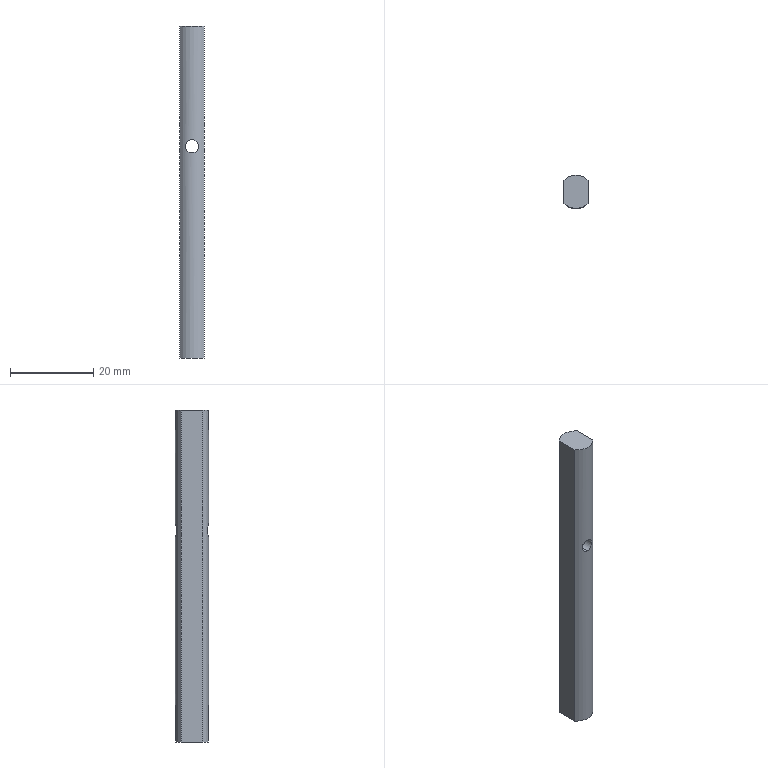Part | STEP file | 8xs200012 | 1 solid | 8 faces | box 6 x 8 x 80 mm | volume 3378 mm3 | cylinder 4 | plane 4 | commonest cylinder face diameters 3.2 x2 8 x2
STEP:
#1=CARTESIAN_POINT('',(0.,0.,0.));
#2=DIRECTION('',(0.,0.,1.));
#3=DIRECTION('',(1.,0.,0.));
#4=AXIS2_PLACEMENT_3D('',#1,#2,#3);
#5=CARTESIAN_POINT('',(0.,-4.,52.6));
#6=VERTEX_POINT('',#5);
#7=CARTESIAN_POINT('',(0.,4.,52.6));
#8=VERTEX_POINT('',#7);
#9=CARTESIAN_POINT('',(0.,-4.,52.6));
#10=DIRECTION('',(0.,1.,0.));
#11=VECTOR('',#10,1.);
#12=LINE('',#9,#11);
#13=CARTESIAN_POINT('',(0.,-4.,51.));
#14=DIRECTION('',(0.,1.,0.));
#15=DIRECTION('',(0.,0.,1.));
#16=AXIS2_PLACEMENT_3D('',#13,#14,#15);
#17=CYLINDRICAL_SURFACE('',#16,1.6);
#18=CARTESIAN_POINT('',(6.283,0.));
#19=DIRECTION('',(0.,1.));
#20=VECTOR('',#19,1.);
#21=LINE('',#18,#20);
#22=(GEOMETRIC_REPRESENTATION_CONTEXT(2)PARAMETRIC_REPRESENTATION_CONTEXT()REPRESENTATION_CONTEXT('',''));
#23=DEFINITIONAL_REPRESENTATION('',(#21),#22);
#24=PCURVE('',#17,#23);
#25=CARTESIAN_POINT('',(0.,-4.,51.));
#26=DIRECTION('',(0.,1.,0.));
#27=DIRECTION('',(0.,0.,1.));
#28=AXIS2_PLACEMENT_3D('',#25,#26,#27);
#29=CYLINDRICAL_SURFACE('',#28,1.6);
#30=CARTESIAN_POINT('',(0.,0.));
#31=DIRECTION('',(0.,1.));
#32=VECTOR('',#31,1.);
#33=LINE('',#30,#32);
#34=(GEOMETRIC_REPRESENTATION_CONTEXT(2)PARAMETRIC_REPRESENTATION_CONTEXT()REPRESENTATION_CONTEXT('',''));
#35=DEFINITIONAL_REPRESENTATION('',(#33),#34);
#36=PCURVE('',#29,#35);
#37=SURFACE_CURVE('',#12,(#24,#36),.PCURVE_S1.);
#38=EDGE_CURVE('',#6,#8,#37,.T.);
#39=ORIENTED_EDGE('',*,*,#38,.T.);
#40=CARTESIAN_POINT('',(0.,4.,49.4));
#41=VERTEX_POINT('',#40);
#42=CARTESIAN_POINT('',(0.,4.,52.6));
#43=CARTESIAN_POINT('',(-0.1069,4.,52.6));
#44=CARTESIAN_POINT('',(-0.2118,3.996,52.589));
#45=CARTESIAN_POINT('',(-0.4179,3.979,52.548));
#46=CARTESIAN_POINT('',(-0.5202,3.967,52.517));
#47=CARTESIAN_POINT('',(-0.8102,3.922,52.396));
#48=CARTESIAN_POINT('',(-0.9862,3.88,52.277));
#49=CARTESIAN_POINT('',(-1.278,3.793,51.985));
#50=CARTESIAN_POINT('',(-1.396,3.749,51.808));
#51=CARTESIAN_POINT('',(-1.517,3.702,51.52));
#52=CARTESIAN_POINT('',(-1.548,3.688,51.418));
#53=CARTESIAN_POINT('',(-1.59,3.671,51.211));
#54=CARTESIAN_POINT('',(-1.6,3.666,51.107));
#55=CARTESIAN_POINT('',(-1.6,3.666,50.895));
#56=CARTESIAN_POINT('',(-1.589,3.671,50.788));
#57=CARTESIAN_POINT('',(-1.548,3.688,50.582));
#58=CARTESIAN_POINT('',(-1.517,3.701,50.481));
#59=CARTESIAN_POINT('',(-1.436,3.734,50.286));
#60=CARTESIAN_POINT('',(-1.387,3.752,50.195));
#61=CARTESIAN_POINT('',(-1.271,3.793,50.023));
#62=CARTESIAN_POINT('',(-1.204,3.815,49.941));
#63=CARTESIAN_POINT('',(-1.058,3.858,49.795));
#64=CARTESIAN_POINT('',(-0.978,3.88,49.729));
#65=CARTESIAN_POINT('',(-0.8051,3.919,49.613));
#66=CARTESIAN_POINT('',(-0.7118,3.937,49.563));
#67=CARTESIAN_POINT('',(-0.4233,3.982,49.443));
#68=CARTESIAN_POINT('',(-0.2106,4.,49.4));
#69=CARTESIAN_POINT('',(0.,4.,49.4));
#70=B_SPLINE_CURVE_WITH_KNOTS('',3,(#42,#43,#44,#45,#46,#47,#48,#49,#50,#51,#52,#53,#54,#55,#56,#57,#58,#59,#60,#61,#62,#63,#64,#65,#66,#67,#68,#69),.UNSPECIFIED.,.F.,.F.,(4,2,2,2,2,2,2,2,2,2,2,2,2,4),(0.,0.000316,0.000632,0.001264,0.001896,0.002212,0.002528,0.002844,0.00316,0.003476,0.003792,0.004108,0.004424,0.005056),.UNSPECIFIED.);
#71=CARTESIAN_POINT('',(6.283,8.));
#72=CARTESIAN_POINT('',(6.267,8.));
#73=CARTESIAN_POINT('',(6.235,7.999));
#74=CARTESIAN_POINT('',(6.187,7.997));
#75=CARTESIAN_POINT('',(6.139,7.994));
#76=CARTESIAN_POINT('',(6.091,7.989));
#77=CARTESIAN_POINT('',(6.043,7.982));
#78=CARTESIAN_POINT('',(5.995,7.974));
#79=CARTESIAN_POINT('',(5.947,7.965));
#80=CARTESIAN_POINT('',(5.899,7.955));
#81=CARTESIAN_POINT('',(5.852,7.944));
#82=CARTESIAN_POINT('',(5.804,7.932));
#83=CARTESIAN_POINT('',(5.757,7.918));
#84=CARTESIAN_POINT('',(5.709,7.905));
#85=CARTESIAN_POINT('',(5.662,7.89));
#86=CARTESIAN_POINT('',(5.615,7.875));
#87=CARTESIAN_POINT('',(5.568,7.86));
#88=CARTESIAN_POINT('',(5.521,7.844));
#89=CARTESIAN_POINT('',(5.474,7.829));
#90=CARTESIAN_POINT('',(5.427,7.813));
#91=CARTESIAN_POINT('',(5.38,7.797));
#92=CARTESIAN_POINT('',(5.332,7.782));
#93=CARTESIAN_POINT('',(5.285,7.767));
#94=CARTESIAN_POINT('',(5.238,7.753));
#95=CARTESIAN_POINT('',(5.19,7.739));
#96=CARTESIAN_POINT('',(5.143,7.726));
#97=CARTESIAN_POINT('',(5.096,7.714));
#98=CARTESIAN_POINT('',(5.048,7.704));
#99=CARTESIAN_POINT('',(5.,7.694));
#100=CARTESIAN_POINT('',(4.952,7.686));
#101=CARTESIAN_POINT('',(4.904,7.678));
#102=CARTESIAN_POINT('',(4.856,7.673));
#103=CARTESIAN_POINT('',(4.809,7.669));
#104=CARTESIAN_POINT('',(4.761,7.667));
#105=CARTESIAN_POINT('',(4.713,7.666));
#106=CARTESIAN_POINT('',(4.665,7.667));
#107=CARTESIAN_POINT('',(4.617,7.669));
#108=CARTESIAN_POINT('',(4.568,7.673));
#109=CARTESIAN_POINT('',(4.52,7.679));
#110=CARTESIAN_POINT('',(4.472,7.686));
#111=CARTESIAN_POINT('',(4.425,7.694));
#112=CARTESIAN_POINT('',(4.377,7.703));
#113=CARTESIAN_POINT('',(4.329,7.714));
#114=CARTESIAN_POINT('',(4.281,7.726));
#115=CARTESIAN_POINT('',(4.234,7.739));
#116=CARTESIAN_POINT('',(4.186,7.753));
#117=CARTESIAN_POINT('',(4.139,7.767));
#118=CARTESIAN_POINT('',(4.092,7.782));
#119=CARTESIAN_POINT('',(4.045,7.797));
#120=CARTESIAN_POINT('',(3.997,7.813));
#121=CARTESIAN_POINT('',(3.95,7.829));
#122=CARTESIAN_POINT('',(3.903,7.845));
#123=CARTESIAN_POINT('',(3.856,7.86));
#124=CARTESIAN_POINT('',(3.809,7.875));
#125=CARTESIAN_POINT('',(3.762,7.89));
#126=CARTESIAN_POINT('',(3.715,7.905));
#127=CARTESIAN_POINT('',(3.667,7.919));
#128=CARTESIAN_POINT('',(3.62,7.932));
#129=CARTESIAN_POINT('',(3.572,7.944));
#130=CARTESIAN_POINT('',(3.525,7.955));
#131=CARTESIAN_POINT('',(3.477,7.965));
#132=CARTESIAN_POINT('',(3.429,7.974));
#133=CARTESIAN_POINT('',(3.382,7.982));
#134=CARTESIAN_POINT('',(3.334,7.988));
#135=CARTESIAN_POINT('',(3.286,7.993));
#136=CARTESIAN_POINT('',(3.238,7.997));
#137=CARTESIAN_POINT('',(3.19,7.999));
#138=CARTESIAN_POINT('',(3.158,8.));
#139=CARTESIAN_POINT('',(3.142,8.));
#140=B_SPLINE_CURVE_WITH_KNOTS('',3,(#71,#72,#73,#74,#75,#76,#77,#78,#79,#80,#81,#82,#83,#84,#85,#86,#87,#88,#89,#90,#91,#92,#93,#94,#95,#96,#97,#98,#99,#100,#101,#102,#103,#104,#105,#106,#107,#108,#109,#110,#111,#112,#113,#114,#115,#116,#117,#118,#119,#120,#121,#122,#123,#124,#125,#126,#127,#128,#129,#130,#131,#132,#133,#134,#135,#136,#137,#138,#139),.UNSPECIFIED.,.F.,.F.,(4,1,1,1,1,1,1,1,1,1,1,1,1,1,1,1,1,1,1,1,1,1,1,1,1,1,1,1,1,1,1,1,1,1,1,1,1,1,1,1,1,1,1,1,1,1,1,1,1,1,1,1,1,1,1,1,1,1,1,1,1,1,1,1,1,1,4),(0.,0.0000766,0.0001532,0.0002298,0.0003064,0.000383,0.0004596,0.0005362,0.0006128,0.0006894,0.000766,0.0008426,0.0009192,0.0009958,0.001072,0.001149,0.001226,0.001302,0.001379,0.001455,0.001532,0.001609,0.001685,0.001762,0.001838,0.001915,0.001992,0.002068,0.002145,0.002221,0.002298,0.002375,0.002451,0.002528,0.002605,0.002681,0.002758,0.002834,0.002911,0.002988,0.003064,0.003141,0.003217,0.003294,0.003371,0.003447,0.003524,0.0036,0.003677,0.003754,0.00383,0.003907,0.003983,0.00406,0.004137,0.004213,0.00429,0.004366,0.004443,0.00452,0.004596,0.004673,0.004749,0.004826,0.004903,0.004979,0.005056),.QUASI_UNIFORM_KNOTS.);
#141=(GEOMETRIC_REPRESENTATION_CONTEXT(2)PARAMETRIC_REPRESENTATION_CONTEXT()REPRESENTATION_CONTEXT('',''));
#142=DEFINITIONAL_REPRESENTATION('',(#140),#141);
#143=PCURVE('',#17,#142);
#144=CARTESIAN_POINT('',(0.,0.,80.));
#145=DIRECTION('',(0.,0.,-1.));
#146=DIRECTION('',(-1.,0.,0.));
#147=AXIS2_PLACEMENT_3D('',#144,#145,#146);
#148=CYLINDRICAL_SURFACE('',#147,4.);
#149=CARTESIAN_POINT('',(1.571,27.4));
#150=CARTESIAN_POINT('',(1.564,27.4));
#151=CARTESIAN_POINT('',(1.551,27.401));
#152=CARTESIAN_POINT('',(1.532,27.407));
#153=CARTESIAN_POINT('',(1.513,27.416));
#154=CARTESIAN_POINT('',(1.494,27.429));
#155=CARTESIAN_POINT('',(1.476,27.445));
#156=CARTESIAN_POINT('',(1.457,27.465));
#157=CARTESIAN_POINT('',(1.438,27.489));
#158=CARTESIAN_POINT('',(1.42,27.516));
#159=CARTESIAN_POINT('',(1.403,27.546));
#160=CARTESIAN_POINT('',(1.385,27.58));
#161=CARTESIAN_POINT('',(1.368,27.616));
#162=CARTESIAN_POINT('',(1.352,27.656));
#163=CARTESIAN_POINT('',(1.336,27.699));
#164=CARTESIAN_POINT('',(1.32,27.744));
#165=CARTESIAN_POINT('',(1.305,27.792));
#166=CARTESIAN_POINT('',(1.291,27.843));
#167=CARTESIAN_POINT('',(1.277,27.896));
#168=CARTESIAN_POINT('',(1.264,27.952));
#169=CARTESIAN_POINT('',(1.251,28.01));
#170=CARTESIAN_POINT('',(1.239,28.07));
#171=CARTESIAN_POINT('',(1.228,28.133));
#172=CARTESIAN_POINT('',(1.217,28.197));
#173=CARTESIAN_POINT('',(1.208,28.264));
#174=CARTESIAN_POINT('',(1.199,28.332));
#175=CARTESIAN_POINT('',(1.191,28.401));
#176=CARTESIAN_POINT('',(1.183,28.472));
#177=CARTESIAN_POINT('',(1.177,28.545));
#178=CARTESIAN_POINT('',(1.172,28.62));
#179=CARTESIAN_POINT('',(1.167,28.695));
#180=CARTESIAN_POINT('',(1.164,28.77));
#181=CARTESIAN_POINT('',(1.161,28.846));
#182=CARTESIAN_POINT('',(1.16,28.922));
#183=CARTESIAN_POINT('',(1.159,28.999));
#184=CARTESIAN_POINT('',(1.16,29.076));
#185=CARTESIAN_POINT('',(1.161,29.153));
#186=CARTESIAN_POINT('',(1.164,29.23));
#187=CARTESIAN_POINT('',(1.167,29.306));
#188=CARTESIAN_POINT('',(1.172,29.38));
#189=CARTESIAN_POINT('',(1.177,29.454));
#190=CARTESIAN_POINT('',(1.183,29.527));
#191=CARTESIAN_POINT('',(1.191,29.599));
#192=CARTESIAN_POINT('',(1.199,29.669));
#193=CARTESIAN_POINT('',(1.208,29.737));
#194=CARTESIAN_POINT('',(1.217,29.804));
#195=CARTESIAN_POINT('',(1.228,29.868));
#196=CARTESIAN_POINT('',(1.239,29.93));
#197=CARTESIAN_POINT('',(1.251,29.991));
#198=CARTESIAN_POINT('',(1.264,30.049));
#199=CARTESIAN_POINT('',(1.277,30.105));
#200=CARTESIAN_POINT('',(1.291,30.159));
#201=CARTESIAN_POINT('',(1.305,30.209));
#202=CARTESIAN_POINT('',(1.32,30.257));
#203=CARTESIAN_POINT('',(1.336,30.302));
#204=CARTESIAN_POINT('',(1.352,30.345));
#205=CARTESIAN_POINT('',(1.369,30.384));
#206=CARTESIAN_POINT('',(1.386,30.421));
#207=CARTESIAN_POINT('',(1.403,30.455));
#208=CARTESIAN_POINT('',(1.421,30.485));
#209=CARTESIAN_POINT('',(1.439,30.511));
#210=CARTESIAN_POINT('',(1.457,30.535));
#211=CARTESIAN_POINT('',(1.476,30.554));
#212=CARTESIAN_POINT('',(1.494,30.571));
#213=CARTESIAN_POINT('',(1.513,30.584));
#214=CARTESIAN_POINT('',(1.532,30.593));
#215=CARTESIAN_POINT('',(1.552,30.599));
#216=CARTESIAN_POINT('',(1.564,30.6));
#217=CARTESIAN_POINT('',(1.571,30.6));
#218=B_SPLINE_CURVE_WITH_KNOTS('',3,(#149,#150,#151,#152,#153,#154,#155,#156,#157,#158,#159,#160,#161,#162,#163,#164,#165,#166,#167,#168,#169,#170,#171,#172,#173,#174,#175,#176,#177,#178,#179,#180,#181,#182,#183,#184,#185,#186,#187,#188,#189,#190,#191,#192,#193,#194,#195,#196,#197,#198,#199,#200,#201,#202,#203,#204,#205,#206,#207,#208,#209,#210,#211,#212,#213,#214,#215,#216,#217),.UNSPECIFIED.,.F.,.F.,(4,1,1,1,1,1,1,1,1,1,1,1,1,1,1,1,1,1,1,1,1,1,1,1,1,1,1,1,1,1,1,1,1,1,1,1,1,1,1,1,1,1,1,1,1,1,1,1,1,1,1,1,1,1,1,1,1,1,1,1,1,1,1,1,1,1,4),(0.,0.0000766,0.0001532,0.0002298,0.0003064,0.000383,0.0004596,0.0005362,0.0006128,0.0006894,0.000766,0.0008426,0.0009192,0.0009958,0.001072,0.001149,0.001226,0.001302,0.001379,0.001455,0.001532,0.001609,0.001685,0.001762,0.001838,0.001915,0.001992,0.002068,0.002145,0.002221,0.002298,0.002375,0.002451,0.002528,0.002605,0.002681,0.002758,0.002834,0.002911,0.002988,0.003064,0.003141,0.003217,0.003294,0.003371,0.003447,0.003524,0.0036,0.003677,0.003754,0.00383,0.003907,0.003983,0.00406,0.004137,0.004213,0.00429,0.004366,0.004443,0.00452,0.004596,0.004673,0.004749,0.004826,0.004903,0.004979,0.005056),.QUASI_UNIFORM_KNOTS.);
#219=(GEOMETRIC_REPRESENTATION_CONTEXT(2)PARAMETRIC_REPRESENTATION_CONTEXT()REPRESENTATION_CONTEXT('',''));
#220=DEFINITIONAL_REPRESENTATION('',(#218),#219);
#221=PCURVE('',#148,#220);
#222=SURFACE_CURVE('',#70,(#143,#221),.PCURVE_S1.);
#223=EDGE_CURVE('',#8,#41,#222,.T.);
#224=ORIENTED_EDGE('',*,*,#223,.T.);
#225=CARTESIAN_POINT('',(0.,-4.,49.4));
#226=VERTEX_POINT('',#225);
#227=CARTESIAN_POINT('',(0.,-4.,49.4));
#228=DIRECTION('',(0.,1.,0.));
#229=VECTOR('',#228,1.);
#230=LINE('',#227,#229);
#231=CARTESIAN_POINT('',(3.142,0.));
#232=DIRECTION('',(0.,1.));
#233=VECTOR('',#232,1.);
#234=LINE('',#231,#233);
#235=(GEOMETRIC_REPRESENTATION_CONTEXT(2)PARAMETRIC_REPRESENTATION_CONTEXT()REPRESENTATION_CONTEXT('',''));
#236=DEFINITIONAL_REPRESENTATION('',(#234),#235);
#237=PCURVE('',#17,#236);
#238=CARTESIAN_POINT('',(3.142,0.));
#239=DIRECTION('',(0.,1.));
#240=VECTOR('',#239,1.);
#241=LINE('',#238,#240);
#242=(GEOMETRIC_REPRESENTATION_CONTEXT(2)PARAMETRIC_REPRESENTATION_CONTEXT()REPRESENTATION_CONTEXT('',''));
#243=DEFINITIONAL_REPRESENTATION('',(#241),#242);
#244=PCURVE('',#29,#243);
#245=SURFACE_CURVE('',#230,(#237,#244),.PCURVE_S1.);
#246=EDGE_CURVE('',#226,#41,#245,.T.);
#247=ORIENTED_EDGE('',*,*,#246,.F.);
#248=CARTESIAN_POINT('',(0.,-4.,49.4));
#249=CARTESIAN_POINT('',(-0.1052,-4.,49.4));
#250=CARTESIAN_POINT('',(-0.2119,-3.996,49.411));
#251=CARTESIAN_POINT('',(-0.4193,-3.979,49.452));
#252=CARTESIAN_POINT('',(-0.5194,-3.967,49.483));
#253=CARTESIAN_POINT('',(-0.713,-3.937,49.564));
#254=CARTESIAN_POINT('',(-0.8061,-3.919,49.614));
#255=CARTESIAN_POINT('',(-0.9782,-3.88,49.73));
#256=CARTESIAN_POINT('',(-1.058,-3.858,49.796));
#257=CARTESIAN_POINT('',(-1.206,-3.815,49.943));
#258=CARTESIAN_POINT('',(-1.271,-3.793,50.023));
#259=CARTESIAN_POINT('',(-1.387,-3.752,50.195));
#260=CARTESIAN_POINT('',(-1.437,-3.733,50.288));
#261=CARTESIAN_POINT('',(-1.517,-3.701,50.481));
#262=CARTESIAN_POINT('',(-1.548,-3.689,50.581));
#263=CARTESIAN_POINT('',(-1.589,-3.671,50.787));
#264=CARTESIAN_POINT('',(-1.6,-3.666,50.894));
#265=CARTESIAN_POINT('',(-1.6,-3.666,51.211));
#266=CARTESIAN_POINT('',(-1.557,-3.685,51.423));
#267=CARTESIAN_POINT('',(-1.437,-3.733,51.712));
#268=CARTESIAN_POINT('',(-1.387,-3.752,51.805));
#269=CARTESIAN_POINT('',(-1.271,-3.793,51.978));
#270=CARTESIAN_POINT('',(-1.205,-3.815,52.057));
#271=CARTESIAN_POINT('',(-1.059,-3.858,52.204));
#272=CARTESIAN_POINT('',(-0.9774,-3.88,52.271));
#273=CARTESIAN_POINT('',(-0.8055,-3.919,52.386));
#274=CARTESIAN_POINT('',(-0.7141,-3.937,52.436));
#275=CARTESIAN_POINT('',(-0.4218,-3.983,52.558));
#276=CARTESIAN_POINT('',(-0.2137,-4.,52.6));
#277=CARTESIAN_POINT('',(0.,-4.,52.6));
#278=B_SPLINE_CURVE_WITH_KNOTS('',3,(#248,#249,#250,#251,#252,#253,#254,#255,#256,#257,#258,#259,#260,#261,#262,#263,#264,#265,#266,#267,#268,#269,#270,#271,#272,#273,#274,#275,#276,#277),.UNSPECIFIED.,.F.,.F.,(4,2,2,2,2,2,2,2,2,2,2,2,2,2,4),(0.005056,0.005372,0.005687,0.006003,0.006319,0.006635,0.006951,0.007266,0.007582,0.008214,0.008529,0.008845,0.009161,0.009477,0.01011),.UNSPECIFIED.);
#279=CARTESIAN_POINT('',(3.142,0.));
#280=CARTESIAN_POINT('',(3.158,0.));
#281=CARTESIAN_POINT('',(3.19,0.0005013));
#282=CARTESIAN_POINT('',(3.238,0.00273));
#283=CARTESIAN_POINT('',(3.286,0.006405));
#284=CARTESIAN_POINT('',(3.334,0.01151));
#285=CARTESIAN_POINT('',(3.382,0.01798));
#286=CARTESIAN_POINT('',(3.43,0.02573));
#287=CARTESIAN_POINT('',(3.477,0.03471));
#288=CARTESIAN_POINT('',(3.525,0.04485));
#289=CARTESIAN_POINT('',(3.573,0.05611));
#290=CARTESIAN_POINT('',(3.62,0.06838));
#291=CARTESIAN_POINT('',(3.668,0.0815));
#292=CARTESIAN_POINT('',(3.715,0.09534));
#293=CARTESIAN_POINT('',(3.763,0.1097));
#294=CARTESIAN_POINT('',(3.81,0.1247));
#295=CARTESIAN_POINT('',(3.857,0.14));
#296=CARTESIAN_POINT('',(3.904,0.1556));
#297=CARTESIAN_POINT('',(3.951,0.1715));
#298=CARTESIAN_POINT('',(3.999,0.1872));
#299=CARTESIAN_POINT('',(4.046,0.2028));
#300=CARTESIAN_POINT('',(4.092,0.218));
#301=CARTESIAN_POINT('',(4.139,0.2328));
#302=CARTESIAN_POINT('',(4.187,0.2472));
#303=CARTESIAN_POINT('',(4.234,0.2609));
#304=CARTESIAN_POINT('',(4.282,0.2738));
#305=CARTESIAN_POINT('',(4.329,0.2857));
#306=CARTESIAN_POINT('',(4.377,0.2965));
#307=CARTESIAN_POINT('',(4.424,0.3061));
#308=CARTESIAN_POINT('',(4.472,0.3144));
#309=CARTESIAN_POINT('',(4.519,0.3214));
#310=CARTESIAN_POINT('',(4.568,0.3269));
#311=CARTESIAN_POINT('',(4.616,0.3309));
#312=CARTESIAN_POINT('',(4.664,0.3334));
#313=CARTESIAN_POINT('',(4.712,0.3342));
#314=CARTESIAN_POINT('',(4.76,0.3334));
#315=CARTESIAN_POINT('',(4.808,0.3309));
#316=CARTESIAN_POINT('',(4.856,0.3268));
#317=CARTESIAN_POINT('',(4.904,0.3213));
#318=CARTESIAN_POINT('',(4.952,0.3143));
#319=CARTESIAN_POINT('',(5.,0.306));
#320=CARTESIAN_POINT('',(5.048,0.2964));
#321=CARTESIAN_POINT('',(5.095,0.2857));
#322=CARTESIAN_POINT('',(5.143,0.2738));
#323=CARTESIAN_POINT('',(5.191,0.2609));
#324=CARTESIAN_POINT('',(5.238,0.2471));
#325=CARTESIAN_POINT('',(5.286,0.2327));
#326=CARTESIAN_POINT('',(5.333,0.2178));
#327=CARTESIAN_POINT('',(5.38,0.2026));
#328=CARTESIAN_POINT('',(5.427,0.1871));
#329=CARTESIAN_POINT('',(5.474,0.1714));
#330=CARTESIAN_POINT('',(5.521,0.1556));
#331=CARTESIAN_POINT('',(5.568,0.1399));
#332=CARTESIAN_POINT('',(5.616,0.1245));
#333=CARTESIAN_POINT('',(5.663,0.1096));
#334=CARTESIAN_POINT('',(5.71,0.09517));
#335=CARTESIAN_POINT('',(5.757,0.08144));
#336=CARTESIAN_POINT('',(5.804,0.06843));
#337=CARTESIAN_POINT('',(5.852,0.05623));
#338=CARTESIAN_POINT('',(5.9,0.0449));
#339=CARTESIAN_POINT('',(5.947,0.03471));
#340=CARTESIAN_POINT('',(5.995,0.02572));
#341=CARTESIAN_POINT('',(6.043,0.01799));
#342=CARTESIAN_POINT('',(6.091,0.01155));
#343=CARTESIAN_POINT('',(6.139,0.006464));
#344=CARTESIAN_POINT('',(6.187,0.002767));
#345=CARTESIAN_POINT('',(6.235,0.0005118));
#346=CARTESIAN_POINT('',(6.267,0.));
#347=CARTESIAN_POINT('',(6.283,0.));
#348=B_SPLINE_CURVE_WITH_KNOTS('',3,(#279,#280,#281,#282,#283,#284,#285,#286,#287,#288,#289,#290,#291,#292,#293,#294,#295,#296,#297,#298,#299,#300,#301,#302,#303,#304,#305,#306,#307,#308,#309,#310,#311,#312,#313,#314,#315,#316,#317,#318,#319,#320,#321,#322,#323,#324,#325,#326,#327,#328,#329,#330,#331,#332,#333,#334,#335,#336,#337,#338,#339,#340,#341,#342,#343,#344,#345,#346,#347),.UNSPECIFIED.,.F.,.F.,(4,1,1,1,1,1,1,1,1,1,1,1,1,1,1,1,1,1,1,1,1,1,1,1,1,1,1,1,1,1,1,1,1,1,1,1,1,1,1,1,1,1,1,1,1,1,1,1,1,1,1,1,1,1,1,1,1,1,1,1,1,1,1,1,1,1,4),(0.005056,0.005132,0.005209,0.005285,0.005362,0.005439,0.005515,0.005592,0.005668,0.005745,0.005821,0.005898,0.005974,0.006051,0.006128,0.006204,0.006281,0.006357,0.006434,0.00651,0.006587,0.006663,0.00674,0.006817,0.006893,0.00697,0.007046,0.007123,0.007199,0.007276,0.007352,0.007429,0.007506,0.007582,0.007659,0.007735,0.007812,0.007888,0.007965,0.008041,0.008118,0.008195,0.008271,0.008348,0.008424,0.008501,0.008577,0.008654,0.00873,0.008807,0.008883,0.00896,0.009037,0.009113,0.00919,0.009266,0.009343,0.009419,0.009496,0.009572,0.009649,0.009726,0.009802,0.009879,0.009955,0.01003,0.01011),.QUASI_UNIFORM_KNOTS.);
#349=(GEOMETRIC_REPRESENTATION_CONTEXT(2)PARAMETRIC_REPRESENTATION_CONTEXT()REPRESENTATION_CONTEXT('',''));
#350=DEFINITIONAL_REPRESENTATION('',(#348),#349);
#351=PCURVE('',#17,#350);
#352=CARTESIAN_POINT('',(0.,0.,80.));
#353=DIRECTION('',(0.,0.,-1.));
#354=DIRECTION('',(-1.,0.,0.));
#355=AXIS2_PLACEMENT_3D('',#352,#353,#354);
#356=CYLINDRICAL_SURFACE('',#355,4.);
#357=CARTESIAN_POINT('',(4.712,30.6));
#358=CARTESIAN_POINT('',(4.719,30.6));
#359=CARTESIAN_POINT('',(4.732,30.599));
#360=CARTESIAN_POINT('',(4.751,30.593));
#361=CARTESIAN_POINT('',(4.77,30.584));
#362=CARTESIAN_POINT('',(4.789,30.571));
#363=CARTESIAN_POINT('',(4.808,30.555));
#364=CARTESIAN_POINT('',(4.826,30.535));
#365=CARTESIAN_POINT('',(4.845,30.511));
#366=CARTESIAN_POINT('',(4.863,30.484));
#367=CARTESIAN_POINT('',(4.88,30.454));
#368=CARTESIAN_POINT('',(4.898,30.421));
#369=CARTESIAN_POINT('',(4.915,30.384));
#370=CARTESIAN_POINT('',(4.931,30.344));
#371=CARTESIAN_POINT('',(4.947,30.302));
#372=CARTESIAN_POINT('',(4.963,30.257));
#373=CARTESIAN_POINT('',(4.978,30.208));
#374=CARTESIAN_POINT('',(4.992,30.158));
#375=CARTESIAN_POINT('',(5.006,30.104));
#376=CARTESIAN_POINT('',(5.02,30.048));
#377=CARTESIAN_POINT('',(5.032,29.99));
#378=CARTESIAN_POINT('',(5.044,29.93));
#379=CARTESIAN_POINT('',(5.055,29.868));
#380=CARTESIAN_POINT('',(5.066,29.803));
#381=CARTESIAN_POINT('',(5.076,29.736));
#382=CARTESIAN_POINT('',(5.085,29.668));
#383=CARTESIAN_POINT('',(5.093,29.598));
#384=CARTESIAN_POINT('',(5.1,29.527));
#385=CARTESIAN_POINT('',(5.106,29.455));
#386=CARTESIAN_POINT('',(5.112,29.381));
#387=CARTESIAN_POINT('',(5.116,29.307));
#388=CARTESIAN_POINT('',(5.119,29.231));
#389=CARTESIAN_POINT('',(5.122,29.154));
#390=CARTESIAN_POINT('',(5.124,29.077));
#391=CARTESIAN_POINT('',(5.124,29.));
#392=CARTESIAN_POINT('',(5.124,28.923));
#393=CARTESIAN_POINT('',(5.122,28.847));
#394=CARTESIAN_POINT('',(5.119,28.771));
#395=CARTESIAN_POINT('',(5.116,28.695));
#396=CARTESIAN_POINT('',(5.112,28.62));
#397=CARTESIAN_POINT('',(5.106,28.546));
#398=CARTESIAN_POINT('',(5.1,28.473));
#399=CARTESIAN_POINT('',(5.093,28.402));
#400=CARTESIAN_POINT('',(5.085,28.332));
#401=CARTESIAN_POINT('',(5.076,28.264));
#402=CARTESIAN_POINT('',(5.066,28.197));
#403=CARTESIAN_POINT('',(5.055,28.132));
#404=CARTESIAN_POINT('',(5.044,28.069));
#405=CARTESIAN_POINT('',(5.032,28.009));
#406=CARTESIAN_POINT('',(5.02,27.951));
#407=CARTESIAN_POINT('',(5.006,27.896));
#408=CARTESIAN_POINT('',(4.992,27.842));
#409=CARTESIAN_POINT('',(4.978,27.791));
#410=CARTESIAN_POINT('',(4.963,27.743));
#411=CARTESIAN_POINT('',(4.947,27.698));
#412=CARTESIAN_POINT('',(4.931,27.655));
#413=CARTESIAN_POINT('',(4.915,27.616));
#414=CARTESIAN_POINT('',(4.898,27.58));
#415=CARTESIAN_POINT('',(4.881,27.546));
#416=CARTESIAN_POINT('',(4.863,27.516));
#417=CARTESIAN_POINT('',(4.845,27.489));
#418=CARTESIAN_POINT('',(4.826,27.465));
#419=CARTESIAN_POINT('',(4.808,27.445));
#420=CARTESIAN_POINT('',(4.789,27.429));
#421=CARTESIAN_POINT('',(4.77,27.416));
#422=CARTESIAN_POINT('',(4.751,27.407));
#423=CARTESIAN_POINT('',(4.732,27.401));
#424=CARTESIAN_POINT('',(4.719,27.4));
#425=CARTESIAN_POINT('',(4.712,27.4));
#426=B_SPLINE_CURVE_WITH_KNOTS('',3,(#357,#358,#359,#360,#361,#362,#363,#364,#365,#366,#367,#368,#369,#370,#371,#372,#373,#374,#375,#376,#377,#378,#379,#380,#381,#382,#383,#384,#385,#386,#387,#388,#389,#390,#391,#392,#393,#394,#395,#396,#397,#398,#399,#400,#401,#402,#403,#404,#405,#406,#407,#408,#409,#410,#411,#412,#413,#414,#415,#416,#417,#418,#419,#420,#421,#422,#423,#424,#425),.UNSPECIFIED.,.F.,.F.,(4,1,1,1,1,1,1,1,1,1,1,1,1,1,1,1,1,1,1,1,1,1,1,1,1,1,1,1,1,1,1,1,1,1,1,1,1,1,1,1,1,1,1,1,1,1,1,1,1,1,1,1,1,1,1,1,1,1,1,1,1,1,1,1,1,1,4),(0.005056,0.005132,0.005209,0.005285,0.005362,0.005439,0.005515,0.005592,0.005668,0.005745,0.005821,0.005898,0.005974,0.006051,0.006128,0.006204,0.006281,0.006357,0.006434,0.00651,0.006587,0.006663,0.00674,0.006817,0.006893,0.00697,0.007046,0.007123,0.007199,0.007276,0.007352,0.007429,0.007506,0.007582,0.007659,0.007735,0.007812,0.007888,0.007965,0.008041,0.008118,0.008195,0.008271,0.008348,0.008424,0.008501,0.008577,0.008654,0.00873,0.008807,0.008883,0.00896,0.009037,0.009113,0.00919,0.009266,0.009343,0.009419,0.009496,0.009572,0.009649,0.009726,0.009802,0.009879,0.009955,0.01003,0.01011),.QUASI_UNIFORM_KNOTS.);
#427=(GEOMETRIC_REPRESENTATION_CONTEXT(2)PARAMETRIC_REPRESENTATION_CONTEXT()REPRESENTATION_CONTEXT('',''));
#428=DEFINITIONAL_REPRESENTATION('',(#426),#427);
#429=PCURVE('',#356,#428);
#430=SURFACE_CURVE('',#278,(#351,#429),.PCURVE_S1.);
#431=EDGE_CURVE('',#226,#6,#430,.T.);
#432=ORIENTED_EDGE('',*,*,#431,.T.);
#433=EDGE_LOOP('',(#39,#224,#247,#432));
#434=FACE_BOUND('',#433,.F.);
#435=ADVANCED_FACE('',(#434),#17,.F.);
#436=ORIENTED_EDGE('',*,*,#223,.T.);
#437=CARTESIAN_POINT('',(0.,4.,49.4));
#438=CARTESIAN_POINT('',(0.1052,4.,49.4));
#439=CARTESIAN_POINT('',(0.2119,3.996,49.411));
#440=CARTESIAN_POINT('',(0.4193,3.979,49.452));
#441=CARTESIAN_POINT('',(0.5194,3.967,49.483));
#442=CARTESIAN_POINT('',(0.713,3.937,49.564));
#443=CARTESIAN_POINT('',(0.8061,3.919,49.614));
#444=CARTESIAN_POINT('',(0.9782,3.88,49.73));
#445=CARTESIAN_POINT('',(1.058,3.858,49.796));
#446=CARTESIAN_POINT('',(1.206,3.815,49.943));
#447=CARTESIAN_POINT('',(1.271,3.793,50.023));
#448=CARTESIAN_POINT('',(1.387,3.752,50.195));
#449=CARTESIAN_POINT('',(1.437,3.733,50.288));
#450=CARTESIAN_POINT('',(1.517,3.701,50.481));
#451=CARTESIAN_POINT('',(1.548,3.689,50.581));
#452=CARTESIAN_POINT('',(1.589,3.671,50.787));
#453=CARTESIAN_POINT('',(1.6,3.666,50.894));
#454=CARTESIAN_POINT('',(1.6,3.666,51.211));
#455=CARTESIAN_POINT('',(1.557,3.685,51.423));
#456=CARTESIAN_POINT('',(1.437,3.733,51.712));
#457=CARTESIAN_POINT('',(1.387,3.752,51.805));
#458=CARTESIAN_POINT('',(1.271,3.793,51.978));
#459=CARTESIAN_POINT('',(1.205,3.815,52.057));
#460=CARTESIAN_POINT('',(1.059,3.858,52.204));
#461=CARTESIAN_POINT('',(0.9774,3.88,52.271));
#462=CARTESIAN_POINT('',(0.8055,3.919,52.386));
#463=CARTESIAN_POINT('',(0.7141,3.937,52.436));
#464=CARTESIAN_POINT('',(0.4218,3.983,52.558));
#465=CARTESIAN_POINT('',(0.2137,4.,52.6));
#466=CARTESIAN_POINT('',(0.,4.,52.6));
#467=B_SPLINE_CURVE_WITH_KNOTS('',3,(#437,#438,#439,#440,#441,#442,#443,#444,#445,#446,#447,#448,#449,#450,#451,#452,#453,#454,#455,#456,#457,#458,#459,#460,#461,#462,#463,#464,#465,#466),.UNSPECIFIED.,.F.,.F.,(4,2,2,2,2,2,2,2,2,2,2,2,2,2,4),(0.005056,0.005372,0.005687,0.006003,0.006319,0.006635,0.006951,0.007266,0.007582,0.008214,0.008529,0.008845,0.009161,0.009477,0.01011),.UNSPECIFIED.);
#468=CARTESIAN_POINT('',(1.571,30.6));
#469=CARTESIAN_POINT('',(1.577,30.6));
#470=CARTESIAN_POINT('',(1.59,30.599));
#471=CARTESIAN_POINT('',(1.609,30.593));
#472=CARTESIAN_POINT('',(1.628,30.584));
#473=CARTESIAN_POINT('',(1.647,30.571));
#474=CARTESIAN_POINT('',(1.666,30.555));
#475=CARTESIAN_POINT('',(1.685,30.535));
#476=CARTESIAN_POINT('',(1.703,30.511));
#477=CARTESIAN_POINT('',(1.721,30.484));
#478=CARTESIAN_POINT('',(1.739,30.454));
#479=CARTESIAN_POINT('',(1.756,30.421));
#480=CARTESIAN_POINT('',(1.773,30.384));
#481=CARTESIAN_POINT('',(1.79,30.344));
#482=CARTESIAN_POINT('',(1.806,30.302));
#483=CARTESIAN_POINT('',(1.821,30.257));
#484=CARTESIAN_POINT('',(1.836,30.208));
#485=CARTESIAN_POINT('',(1.851,30.158));
#486=CARTESIAN_POINT('',(1.865,30.104));
#487=CARTESIAN_POINT('',(1.878,30.048));
#488=CARTESIAN_POINT('',(1.891,29.99));
#489=CARTESIAN_POINT('',(1.903,29.93));
#490=CARTESIAN_POINT('',(1.914,29.868));
#491=CARTESIAN_POINT('',(1.924,29.803));
#492=CARTESIAN_POINT('',(1.934,29.736));
#493=CARTESIAN_POINT('',(1.943,29.668));
#494=CARTESIAN_POINT('',(1.951,29.598));
#495=CARTESIAN_POINT('',(1.958,29.527));
#496=CARTESIAN_POINT('',(1.965,29.455));
#497=CARTESIAN_POINT('',(1.97,29.381));
#498=CARTESIAN_POINT('',(1.974,29.307));
#499=CARTESIAN_POINT('',(1.978,29.231));
#500=CARTESIAN_POINT('',(1.98,29.154));
#501=CARTESIAN_POINT('',(1.982,29.077));
#502=CARTESIAN_POINT('',(1.982,29.));
#503=CARTESIAN_POINT('',(1.982,28.923));
#504=CARTESIAN_POINT('',(1.98,28.847));
#505=CARTESIAN_POINT('',(1.978,28.771));
#506=CARTESIAN_POINT('',(1.974,28.695));
#507=CARTESIAN_POINT('',(1.97,28.62));
#508=CARTESIAN_POINT('',(1.965,28.546));
#509=CARTESIAN_POINT('',(1.958,28.473));
#510=CARTESIAN_POINT('',(1.951,28.402));
#511=CARTESIAN_POINT('',(1.943,28.332));
#512=CARTESIAN_POINT('',(1.934,28.264));
#513=CARTESIAN_POINT('',(1.924,28.197));
#514=CARTESIAN_POINT('',(1.914,28.132));
#515=CARTESIAN_POINT('',(1.902,28.069));
#516=CARTESIAN_POINT('',(1.89,28.009));
#517=CARTESIAN_POINT('',(1.878,27.951));
#518=CARTESIAN_POINT('',(1.865,27.896));
#519=CARTESIAN_POINT('',(1.851,27.842));
#520=CARTESIAN_POINT('',(1.836,27.791));
#521=CARTESIAN_POINT('',(1.821,27.743));
#522=CARTESIAN_POINT('',(1.806,27.698));
#523=CARTESIAN_POINT('',(1.79,27.655));
#524=CARTESIAN_POINT('',(1.773,27.616));
#525=CARTESIAN_POINT('',(1.756,27.58));
#526=CARTESIAN_POINT('',(1.739,27.546));
#527=CARTESIAN_POINT('',(1.721,27.516));
#528=CARTESIAN_POINT('',(1.703,27.489));
#529=CARTESIAN_POINT('',(1.685,27.465));
#530=CARTESIAN_POINT('',(1.666,27.445));
#531=CARTESIAN_POINT('',(1.647,27.429));
#532=CARTESIAN_POINT('',(1.628,27.416));
#533=CARTESIAN_POINT('',(1.609,27.407));
#534=CARTESIAN_POINT('',(1.59,27.401));
#535=CARTESIAN_POINT('',(1.577,27.4));
#536=CARTESIAN_POINT('',(1.571,27.4));
#537=B_SPLINE_CURVE_WITH_KNOTS('',3,(#468,#469,#470,#471,#472,#473,#474,#475,#476,#477,#478,#479,#480,#481,#482,#483,#484,#485,#486,#487,#488,#489,#490,#491,#492,#493,#494,#495,#496,#497,#498,#499,#500,#501,#502,#503,#504,#505,#506,#507,#508,#509,#510,#511,#512,#513,#514,#515,#516,#517,#518,#519,#520,#521,#522,#523,#524,#525,#526,#527,#528,#529,#530,#531,#532,#533,#534,#535,#536),.UNSPECIFIED.,.F.,.F.,(4,1,1,1,1,1,1,1,1,1,1,1,1,1,1,1,1,1,1,1,1,1,1,1,1,1,1,1,1,1,1,1,1,1,1,1,1,1,1,1,1,1,1,1,1,1,1,1,1,1,1,1,1,1,1,1,1,1,1,1,1,1,1,1,1,1,4),(0.005056,0.005132,0.005209,0.005285,0.005362,0.005439,0.005515,0.005592,0.005668,0.005745,0.005821,0.005898,0.005974,0.006051,0.006128,0.006204,0.006281,0.006357,0.006434,0.00651,0.006587,0.006663,0.00674,0.006817,0.006893,0.00697,0.007046,0.007123,0.007199,0.007276,0.007352,0.007429,0.007506,0.007582,0.007659,0.007735,0.007812,0.007888,0.007965,0.008041,0.008118,0.008195,0.008271,0.008348,0.008424,0.008501,0.008577,0.008654,0.00873,0.008807,0.008883,0.00896,0.009037,0.009113,0.00919,0.009266,0.009343,0.009419,0.009496,0.009572,0.009649,0.009726,0.009802,0.009879,0.009955,0.01003,0.01011),.QUASI_UNIFORM_KNOTS.);
#538=(GEOMETRIC_REPRESENTATION_CONTEXT(2)PARAMETRIC_REPRESENTATION_CONTEXT()REPRESENTATION_CONTEXT('',''));
#539=DEFINITIONAL_REPRESENTATION('',(#537),#538);
#540=PCURVE('',#148,#539);
#541=CARTESIAN_POINT('',(3.142,8.));
#542=CARTESIAN_POINT('',(3.126,8.));
#543=CARTESIAN_POINT('',(3.094,7.999));
#544=CARTESIAN_POINT('',(3.045,7.997));
#545=CARTESIAN_POINT('',(2.997,7.994));
#546=CARTESIAN_POINT('',(2.949,7.988));
#547=CARTESIAN_POINT('',(2.901,7.982));
#548=CARTESIAN_POINT('',(2.853,7.974));
#549=CARTESIAN_POINT('',(2.806,7.965));
#550=CARTESIAN_POINT('',(2.758,7.955));
#551=CARTESIAN_POINT('',(2.71,7.944));
#552=CARTESIAN_POINT('',(2.663,7.932));
#553=CARTESIAN_POINT('',(2.615,7.918));
#554=CARTESIAN_POINT('',(2.568,7.905));
#555=CARTESIAN_POINT('',(2.521,7.89));
#556=CARTESIAN_POINT('',(2.474,7.875));
#557=CARTESIAN_POINT('',(2.426,7.86));
#558=CARTESIAN_POINT('',(2.379,7.844));
#559=CARTESIAN_POINT('',(2.332,7.828));
#560=CARTESIAN_POINT('',(2.285,7.813));
#561=CARTESIAN_POINT('',(2.238,7.797));
#562=CARTESIAN_POINT('',(2.191,7.782));
#563=CARTESIAN_POINT('',(2.144,7.767));
#564=CARTESIAN_POINT('',(2.096,7.753));
#565=CARTESIAN_POINT('',(2.049,7.739));
#566=CARTESIAN_POINT('',(2.001,7.726));
#567=CARTESIAN_POINT('',(1.954,7.714));
#568=CARTESIAN_POINT('',(1.906,7.704));
#569=CARTESIAN_POINT('',(1.859,7.694));
#570=CARTESIAN_POINT('',(1.811,7.686));
#571=CARTESIAN_POINT('',(1.764,7.679));
#572=CARTESIAN_POINT('',(1.716,7.673));
#573=CARTESIAN_POINT('',(1.667,7.669));
#574=CARTESIAN_POINT('',(1.619,7.667));
#575=CARTESIAN_POINT('',(1.571,7.666));
#576=CARTESIAN_POINT('',(1.523,7.667));
#577=CARTESIAN_POINT('',(1.475,7.669));
#578=CARTESIAN_POINT('',(1.427,7.673));
#579=CARTESIAN_POINT('',(1.379,7.679));
#580=CARTESIAN_POINT('',(1.331,7.686));
#581=CARTESIAN_POINT('',(1.283,7.694));
#582=CARTESIAN_POINT('',(1.235,7.704));
#583=CARTESIAN_POINT('',(1.188,7.714));
#584=CARTESIAN_POINT('',(1.14,7.726));
#585=CARTESIAN_POINT('',(1.093,7.739));
#586=CARTESIAN_POINT('',(1.045,7.753));
#587=CARTESIAN_POINT('',(0.9976,7.767));
#588=CARTESIAN_POINT('',(0.9504,7.782));
#589=CARTESIAN_POINT('',(0.9034,7.797));
#590=CARTESIAN_POINT('',(0.8564,7.813));
#591=CARTESIAN_POINT('',(0.8094,7.829));
#592=CARTESIAN_POINT('',(0.7623,7.844));
#593=CARTESIAN_POINT('',(0.7149,7.86));
#594=CARTESIAN_POINT('',(0.6676,7.875));
#595=CARTESIAN_POINT('',(0.6203,7.89));
#596=CARTESIAN_POINT('',(0.5733,7.905));
#597=CARTESIAN_POINT('',(0.5263,7.919));
#598=CARTESIAN_POINT('',(0.479,7.932));
#599=CARTESIAN_POINT('',(0.4316,7.944));
#600=CARTESIAN_POINT('',(0.3836,7.955));
#601=CARTESIAN_POINT('',(0.3357,7.965));
#602=CARTESIAN_POINT('',(0.288,7.974));
#603=CARTESIAN_POINT('',(0.2402,7.982));
#604=CARTESIAN_POINT('',(0.1924,7.988));
#605=CARTESIAN_POINT('',(0.1446,7.994));
#606=CARTESIAN_POINT('',(0.09663,7.997));
#607=CARTESIAN_POINT('',(0.04847,7.999));
#608=CARTESIAN_POINT('',(0.01619,8.));
#609=CARTESIAN_POINT('',(0.,8.));
#610=B_SPLINE_CURVE_WITH_KNOTS('',3,(#541,#542,#543,#544,#545,#546,#547,#548,#549,#550,#551,#552,#553,#554,#555,#556,#557,#558,#559,#560,#561,#562,#563,#564,#565,#566,#567,#568,#569,#570,#571,#572,#573,#574,#575,#576,#577,#578,#579,#580,#581,#582,#583,#584,#585,#586,#587,#588,#589,#590,#591,#592,#593,#594,#595,#596,#597,#598,#599,#600,#601,#602,#603,#604,#605,#606,#607,#608,#609),.UNSPECIFIED.,.F.,.F.,(4,1,1,1,1,1,1,1,1,1,1,1,1,1,1,1,1,1,1,1,1,1,1,1,1,1,1,1,1,1,1,1,1,1,1,1,1,1,1,1,1,1,1,1,1,1,1,1,1,1,1,1,1,1,1,1,1,1,1,1,1,1,1,1,1,1,4),(0.005056,0.005132,0.005209,0.005285,0.005362,0.005439,0.005515,0.005592,0.005668,0.005745,0.005821,0.005898,0.005974,0.006051,0.006128,0.006204,0.006281,0.006357,0.006434,0.00651,0.006587,0.006663,0.00674,0.006817,0.006893,0.00697,0.007046,0.007123,0.007199,0.007276,0.007352,0.007429,0.007506,0.007582,0.007659,0.007735,0.007812,0.007888,0.007965,0.008041,0.008118,0.008195,0.008271,0.008348,0.008424,0.008501,0.008577,0.008654,0.00873,0.008807,0.008883,0.00896,0.009037,0.009113,0.00919,0.009266,0.009343,0.009419,0.009496,0.009572,0.009649,0.009726,0.009802,0.009879,0.009955,0.01003,0.01011),.QUASI_UNIFORM_KNOTS.);
#611=(GEOMETRIC_REPRESENTATION_CONTEXT(2)PARAMETRIC_REPRESENTATION_CONTEXT()REPRESENTATION_CONTEXT('',''));
#612=DEFINITIONAL_REPRESENTATION('',(#610),#611);
#613=PCURVE('',#29,#612);
#614=SURFACE_CURVE('',#467,(#540,#613),.PCURVE_S1.);
#615=EDGE_CURVE('',#41,#8,#614,.T.);
#616=ORIENTED_EDGE('',*,*,#615,.T.);
#617=EDGE_LOOP('',(#436,#616));
#618=FACE_BOUND('',#617,.T.);
#619=CARTESIAN_POINT('',(3.,2.646,0.));
#620=VERTEX_POINT('',#619);
#621=CARTESIAN_POINT('',(-3.,2.646,0.));
#622=VERTEX_POINT('',#621);
#623=CARTESIAN_POINT('',(0.,0.,0.));
#624=DIRECTION('',(0.,0.,1.));
#625=DIRECTION('',(1.,0.,0.));
#626=AXIS2_PLACEMENT_3D('',#623,#624,#625);
#627=CIRCLE('',#626,4.);
#628=CARTESIAN_POINT('',(3.142,80.));
#629=DIRECTION('',(-1.,0.));
#630=VECTOR('',#629,1.);
#631=LINE('',#628,#630);
#632=(GEOMETRIC_REPRESENTATION_CONTEXT(2)PARAMETRIC_REPRESENTATION_CONTEXT()REPRESENTATION_CONTEXT('',''));
#633=DEFINITIONAL_REPRESENTATION('',(#631),#632);
#634=PCURVE('',#148,#633);
#635=CARTESIAN_POINT('',(0.,0.,0.));
#636=DIRECTION('',(0.,0.,1.));
#637=DIRECTION('',(1.,0.,0.));
#638=AXIS2_PLACEMENT_3D('',#635,#636,#637);
#639=PLANE('',#638);
#640=CARTESIAN_POINT('',(0.,0.));
#641=DIRECTION('',(1.,0.));
#642=AXIS2_PLACEMENT_2D('',#640,#641);
#643=CIRCLE('',#642,4.);
#644=(GEOMETRIC_REPRESENTATION_CONTEXT(2)PARAMETRIC_REPRESENTATION_CONTEXT()REPRESENTATION_CONTEXT('',''));
#645=DEFINITIONAL_REPRESENTATION('',(#643),#644);
#646=PCURVE('',#639,#645);
#647=SURFACE_CURVE('',#627,(#634,#646),.PCURVE_S1.);
#648=EDGE_CURVE('',#620,#622,#647,.T.);
#649=ORIENTED_EDGE('',*,*,#648,.T.);
#650=CARTESIAN_POINT('',(-3.,2.646,80.));
#651=VERTEX_POINT('',#650);
#652=CARTESIAN_POINT('',(-3.,2.646,80.));
#653=DIRECTION('',(0.,0.,-1.));
#654=VECTOR('',#653,1.);
#655=LINE('',#652,#654);
#656=CARTESIAN_POINT('',(0.7227,0.));
#657=DIRECTION('',(0.,1.));
#658=VECTOR('',#657,1.);
#659=LINE('',#656,#658);
#660=(GEOMETRIC_REPRESENTATION_CONTEXT(2)PARAMETRIC_REPRESENTATION_CONTEXT()REPRESENTATION_CONTEXT('',''));
#661=DEFINITIONAL_REPRESENTATION('',(#659),#660);
#662=PCURVE('',#148,#661);
#663=CARTESIAN_POINT('',(-3.,2.646,80.));
#664=DIRECTION('',(1.,0.,0.));
#665=DIRECTION('',(0.,0.,-1.));
#666=AXIS2_PLACEMENT_3D('',#663,#664,#665);
#667=PLANE('',#666);
#668=CARTESIAN_POINT('',(0.,0.));
#669=DIRECTION('',(1.,0.));
#670=VECTOR('',#669,1.);
#671=LINE('',#668,#670);
#672=(GEOMETRIC_REPRESENTATION_CONTEXT(2)PARAMETRIC_REPRESENTATION_CONTEXT()REPRESENTATION_CONTEXT('',''));
#673=DEFINITIONAL_REPRESENTATION('',(#671),#672);
#674=PCURVE('',#667,#673);
#675=SURFACE_CURVE('',#655,(#662,#674),.PCURVE_S1.);
#676=EDGE_CURVE('',#651,#622,#675,.T.);
#677=ORIENTED_EDGE('',*,*,#676,.F.);
#678=CARTESIAN_POINT('',(3.,2.646,80.));
#679=VERTEX_POINT('',#678);
#680=CARTESIAN_POINT('',(0.,0.,80.));
#681=DIRECTION('',(0.,0.,1.));
#682=DIRECTION('',(1.,0.,0.));
#683=AXIS2_PLACEMENT_3D('',#680,#681,#682);
#684=CIRCLE('',#683,4.);
#685=CARTESIAN_POINT('',(3.142,0.));
#686=DIRECTION('',(-1.,0.));
#687=VECTOR('',#686,1.);
#688=LINE('',#685,#687);
#689=(GEOMETRIC_REPRESENTATION_CONTEXT(2)PARAMETRIC_REPRESENTATION_CONTEXT()REPRESENTATION_CONTEXT('',''));
#690=DEFINITIONAL_REPRESENTATION('',(#688),#689);
#691=PCURVE('',#148,#690);
#692=CARTESIAN_POINT('',(0.,0.,80.));
#693=DIRECTION('',(0.,0.,1.));
#694=DIRECTION('',(1.,0.,0.));
#695=AXIS2_PLACEMENT_3D('',#692,#693,#694);
#696=PLANE('',#695);
#697=CARTESIAN_POINT('',(0.,0.));
#698=DIRECTION('',(1.,0.));
#699=AXIS2_PLACEMENT_2D('',#697,#698);
#700=CIRCLE('',#699,4.);
#701=(GEOMETRIC_REPRESENTATION_CONTEXT(2)PARAMETRIC_REPRESENTATION_CONTEXT()REPRESENTATION_CONTEXT('',''));
#702=DEFINITIONAL_REPRESENTATION('',(#700),#701);
#703=PCURVE('',#696,#702);
#704=SURFACE_CURVE('',#684,(#691,#703),.PCURVE_S1.);
#705=EDGE_CURVE('',#679,#651,#704,.T.);
#706=ORIENTED_EDGE('',*,*,#705,.F.);
#707=CARTESIAN_POINT('',(3.,2.646,80.));
#708=DIRECTION('',(0.,0.,-1.));
#709=VECTOR('',#708,1.);
#710=LINE('',#707,#709);
#711=CARTESIAN_POINT('',(2.419,0.));
#712=DIRECTION('',(0.,1.));
#713=VECTOR('',#712,1.);
#714=LINE('',#711,#713);
#715=(GEOMETRIC_REPRESENTATION_CONTEXT(2)PARAMETRIC_REPRESENTATION_CONTEXT()REPRESENTATION_CONTEXT('',''));
#716=DEFINITIONAL_REPRESENTATION('',(#714),#715);
#717=PCURVE('',#148,#716);
#718=CARTESIAN_POINT('',(3.,2.646,80.));
#719=DIRECTION('',(-1.,0.,0.));
#720=DIRECTION('',(0.,0.,1.));
#721=AXIS2_PLACEMENT_3D('',#718,#719,#720);
#722=PLANE('',#721);
#723=CARTESIAN_POINT('',(0.,0.));
#724=DIRECTION('',(-1.,0.));
#725=VECTOR('',#724,1.);
#726=LINE('',#723,#725);
#727=(GEOMETRIC_REPRESENTATION_CONTEXT(2)PARAMETRIC_REPRESENTATION_CONTEXT()REPRESENTATION_CONTEXT('',''));
#728=DEFINITIONAL_REPRESENTATION('',(#726),#727);
#729=PCURVE('',#722,#728);
#730=SURFACE_CURVE('',#710,(#717,#729),.PCURVE_S1.);
#731=EDGE_CURVE('',#679,#620,#730,.T.);
#732=ORIENTED_EDGE('',*,*,#731,.T.);
#733=EDGE_LOOP('',(#649,#677,#706,#732));
#734=FACE_BOUND('',#733,.T.);
#735=ADVANCED_FACE('',(#618,#734),#148,.T.);
#736=CARTESIAN_POINT('',(-3.,-2.646,0.));
#737=VERTEX_POINT('',#736);
#738=CARTESIAN_POINT('',(-3.,2.646,0.));
#739=DIRECTION('',(0.,-1.,0.));
#740=VECTOR('',#739,1.);
#741=LINE('',#738,#740);
#742=CARTESIAN_POINT('',(80.,0.));
#743=DIRECTION('',(0.,-1.));
#744=VECTOR('',#743,1.);
#745=LINE('',#742,#744);
#746=(GEOMETRIC_REPRESENTATION_CONTEXT(2)PARAMETRIC_REPRESENTATION_CONTEXT()REPRESENTATION_CONTEXT('',''));
#747=DEFINITIONAL_REPRESENTATION('',(#745),#746);
#748=PCURVE('',#667,#747);
#749=CARTESIAN_POINT('',(-3.,2.646));
#750=DIRECTION('',(0.,-1.));
#751=VECTOR('',#750,1.);
#752=LINE('',#749,#751);
#753=(GEOMETRIC_REPRESENTATION_CONTEXT(2)PARAMETRIC_REPRESENTATION_CONTEXT()REPRESENTATION_CONTEXT('',''));
#754=DEFINITIONAL_REPRESENTATION('',(#752),#753);
#755=PCURVE('',#639,#754);
#756=SURFACE_CURVE('',#741,(#748,#755),.PCURVE_S1.);
#757=EDGE_CURVE('',#622,#737,#756,.T.);
#758=ORIENTED_EDGE('',*,*,#757,.T.);
#759=CARTESIAN_POINT('',(-3.,-2.646,80.));
#760=VERTEX_POINT('',#759);
#761=CARTESIAN_POINT('',(-3.,-2.646,80.));
#762=DIRECTION('',(0.,0.,-1.));
#763=VECTOR('',#762,1.);
#764=LINE('',#761,#763);
#765=CARTESIAN_POINT('',(0.,-5.292));
#766=DIRECTION('',(1.,0.));
#767=VECTOR('',#766,1.);
#768=LINE('',#765,#767);
#769=(GEOMETRIC_REPRESENTATION_CONTEXT(2)PARAMETRIC_REPRESENTATION_CONTEXT()REPRESENTATION_CONTEXT('',''));
#770=DEFINITIONAL_REPRESENTATION('',(#768),#769);
#771=PCURVE('',#667,#770);
#772=CARTESIAN_POINT('',(5.56,0.));
#773=DIRECTION('',(0.,1.));
#774=VECTOR('',#773,1.);
#775=LINE('',#772,#774);
#776=(GEOMETRIC_REPRESENTATION_CONTEXT(2)PARAMETRIC_REPRESENTATION_CONTEXT()REPRESENTATION_CONTEXT('',''));
#777=DEFINITIONAL_REPRESENTATION('',(#775),#776);
#778=PCURVE('',#356,#777);
#779=SURFACE_CURVE('',#764,(#771,#778),.PCURVE_S1.);
#780=EDGE_CURVE('',#760,#737,#779,.T.);
#781=ORIENTED_EDGE('',*,*,#780,.F.);
#782=CARTESIAN_POINT('',(-3.,2.646,80.));
#783=DIRECTION('',(0.,-1.,0.));
#784=VECTOR('',#783,1.);
#785=LINE('',#782,#784);
#786=CARTESIAN_POINT('',(0.,0.));
#787=DIRECTION('',(0.,-1.));
#788=VECTOR('',#787,1.);
#789=LINE('',#786,#788);
#790=(GEOMETRIC_REPRESENTATION_CONTEXT(2)PARAMETRIC_REPRESENTATION_CONTEXT()REPRESENTATION_CONTEXT('',''));
#791=DEFINITIONAL_REPRESENTATION('',(#789),#790);
#792=PCURVE('',#667,#791);
#793=CARTESIAN_POINT('',(-3.,2.646));
#794=DIRECTION('',(0.,-1.));
#795=VECTOR('',#794,1.);
#796=LINE('',#793,#795);
#797=(GEOMETRIC_REPRESENTATION_CONTEXT(2)PARAMETRIC_REPRESENTATION_CONTEXT()REPRESENTATION_CONTEXT('',''));
#798=DEFINITIONAL_REPRESENTATION('',(#796),#797);
#799=PCURVE('',#696,#798);
#800=SURFACE_CURVE('',#785,(#792,#799),.PCURVE_S1.);
#801=EDGE_CURVE('',#651,#760,#800,.T.);
#802=ORIENTED_EDGE('',*,*,#801,.F.);
#803=ORIENTED_EDGE('',*,*,#676,.T.);
#804=EDGE_LOOP('',(#758,#781,#802,#803));
#805=FACE_BOUND('',#804,.T.);
#806=ADVANCED_FACE('',(#805),#667,.F.);
#807=CARTESIAN_POINT('',(0.,-4.,52.6));
#808=CARTESIAN_POINT('',(0.1069,-4.,52.6));
#809=CARTESIAN_POINT('',(0.2118,-3.996,52.589));
#810=CARTESIAN_POINT('',(0.4179,-3.979,52.548));
#811=CARTESIAN_POINT('',(0.5202,-3.967,52.517));
#812=CARTESIAN_POINT('',(0.8102,-3.922,52.396));
#813=CARTESIAN_POINT('',(0.9862,-3.88,52.277));
#814=CARTESIAN_POINT('',(1.278,-3.793,51.985));
#815=CARTESIAN_POINT('',(1.396,-3.749,51.808));
#816=CARTESIAN_POINT('',(1.517,-3.702,51.52));
#817=CARTESIAN_POINT('',(1.548,-3.688,51.418));
#818=CARTESIAN_POINT('',(1.59,-3.671,51.211));
#819=CARTESIAN_POINT('',(1.6,-3.666,51.107));
#820=CARTESIAN_POINT('',(1.6,-3.666,50.895));
#821=CARTESIAN_POINT('',(1.589,-3.671,50.788));
#822=CARTESIAN_POINT('',(1.548,-3.688,50.582));
#823=CARTESIAN_POINT('',(1.517,-3.701,50.481));
#824=CARTESIAN_POINT('',(1.436,-3.734,50.286));
#825=CARTESIAN_POINT('',(1.387,-3.752,50.195));
#826=CARTESIAN_POINT('',(1.271,-3.793,50.023));
#827=CARTESIAN_POINT('',(1.204,-3.815,49.941));
#828=CARTESIAN_POINT('',(1.058,-3.858,49.795));
#829=CARTESIAN_POINT('',(0.978,-3.88,49.729));
#830=CARTESIAN_POINT('',(0.8051,-3.919,49.613));
#831=CARTESIAN_POINT('',(0.7118,-3.937,49.563));
#832=CARTESIAN_POINT('',(0.4233,-3.982,49.443));
#833=CARTESIAN_POINT('',(0.2106,-4.,49.4));
#834=CARTESIAN_POINT('',(0.,-4.,49.4));
#835=B_SPLINE_CURVE_WITH_KNOTS('',3,(#807,#808,#809,#810,#811,#812,#813,#814,#815,#816,#817,#818,#819,#820,#821,#822,#823,#824,#825,#826,#827,#828,#829,#830,#831,#832,#833,#834),.UNSPECIFIED.,.F.,.F.,(4,2,2,2,2,2,2,2,2,2,2,2,2,4),(0.,0.000316,0.000632,0.001264,0.001896,0.002212,0.002528,0.002844,0.00316,0.003476,0.003792,0.004108,0.004424,0.005056),.UNSPECIFIED.);
#836=CARTESIAN_POINT('',(4.712,27.4));
#837=CARTESIAN_POINT('',(4.706,27.4));
#838=CARTESIAN_POINT('',(4.693,27.401));
#839=CARTESIAN_POINT('',(4.674,27.407));
#840=CARTESIAN_POINT('',(4.655,27.416));
#841=CARTESIAN_POINT('',(4.636,27.429));
#842=CARTESIAN_POINT('',(4.617,27.445));
#843=CARTESIAN_POINT('',(4.598,27.465));
#844=CARTESIAN_POINT('',(4.58,27.489));
#845=CARTESIAN_POINT('',(4.562,27.516));
#846=CARTESIAN_POINT('',(4.544,27.546));
#847=CARTESIAN_POINT('',(4.527,27.58));
#848=CARTESIAN_POINT('',(4.51,27.616));
#849=CARTESIAN_POINT('',(4.493,27.656));
#850=CARTESIAN_POINT('',(4.477,27.699));
#851=CARTESIAN_POINT('',(4.462,27.744));
#852=CARTESIAN_POINT('',(4.447,27.792));
#853=CARTESIAN_POINT('',(4.432,27.843));
#854=CARTESIAN_POINT('',(4.419,27.896));
#855=CARTESIAN_POINT('',(4.405,27.952));
#856=CARTESIAN_POINT('',(4.393,28.01));
#857=CARTESIAN_POINT('',(4.381,28.07));
#858=CARTESIAN_POINT('',(4.369,28.133));
#859=CARTESIAN_POINT('',(4.359,28.197));
#860=CARTESIAN_POINT('',(4.349,28.264));
#861=CARTESIAN_POINT('',(4.34,28.332));
#862=CARTESIAN_POINT('',(4.332,28.401));
#863=CARTESIAN_POINT('',(4.325,28.472));
#864=CARTESIAN_POINT('',(4.319,28.545));
#865=CARTESIAN_POINT('',(4.313,28.62));
#866=CARTESIAN_POINT('',(4.309,28.695));
#867=CARTESIAN_POINT('',(4.305,28.77));
#868=CARTESIAN_POINT('',(4.303,28.846));
#869=CARTESIAN_POINT('',(4.301,28.922));
#870=CARTESIAN_POINT('',(4.301,28.999));
#871=CARTESIAN_POINT('',(4.301,29.076));
#872=CARTESIAN_POINT('',(4.303,29.153));
#873=CARTESIAN_POINT('',(4.305,29.23));
#874=CARTESIAN_POINT('',(4.309,29.306));
#875=CARTESIAN_POINT('',(4.313,29.38));
#876=CARTESIAN_POINT('',(4.319,29.454));
#877=CARTESIAN_POINT('',(4.325,29.527));
#878=CARTESIAN_POINT('',(4.332,29.599));
#879=CARTESIAN_POINT('',(4.34,29.669));
#880=CARTESIAN_POINT('',(4.349,29.737));
#881=CARTESIAN_POINT('',(4.359,29.804));
#882=CARTESIAN_POINT('',(4.369,29.868));
#883=CARTESIAN_POINT('',(4.381,29.93));
#884=CARTESIAN_POINT('',(4.393,29.991));
#885=CARTESIAN_POINT('',(4.405,30.049));
#886=CARTESIAN_POINT('',(4.419,30.105));
#887=CARTESIAN_POINT('',(4.433,30.159));
#888=CARTESIAN_POINT('',(4.447,30.209));
#889=CARTESIAN_POINT('',(4.462,30.257));
#890=CARTESIAN_POINT('',(4.478,30.302));
#891=CARTESIAN_POINT('',(4.494,30.345));
#892=CARTESIAN_POINT('',(4.51,30.384));
#893=CARTESIAN_POINT('',(4.527,30.421));
#894=CARTESIAN_POINT('',(4.545,30.455));
#895=CARTESIAN_POINT('',(4.562,30.485));
#896=CARTESIAN_POINT('',(4.58,30.511));
#897=CARTESIAN_POINT('',(4.599,30.535));
#898=CARTESIAN_POINT('',(4.617,30.554));
#899=CARTESIAN_POINT('',(4.636,30.571));
#900=CARTESIAN_POINT('',(4.655,30.584));
#901=CARTESIAN_POINT('',(4.674,30.593));
#902=CARTESIAN_POINT('',(4.693,30.599));
#903=CARTESIAN_POINT('',(4.706,30.6));
#904=CARTESIAN_POINT('',(4.712,30.6));
#905=B_SPLINE_CURVE_WITH_KNOTS('',3,(#836,#837,#838,#839,#840,#841,#842,#843,#844,#845,#846,#847,#848,#849,#850,#851,#852,#853,#854,#855,#856,#857,#858,#859,#860,#861,#862,#863,#864,#865,#866,#867,#868,#869,#870,#871,#872,#873,#874,#875,#876,#877,#878,#879,#880,#881,#882,#883,#884,#885,#886,#887,#888,#889,#890,#891,#892,#893,#894,#895,#896,#897,#898,#899,#900,#901,#902,#903,#904),.UNSPECIFIED.,.F.,.F.,(4,1,1,1,1,1,1,1,1,1,1,1,1,1,1,1,1,1,1,1,1,1,1,1,1,1,1,1,1,1,1,1,1,1,1,1,1,1,1,1,1,1,1,1,1,1,1,1,1,1,1,1,1,1,1,1,1,1,1,1,1,1,1,1,1,1,4),(0.,0.0000766,0.0001532,0.0002298,0.0003064,0.000383,0.0004596,0.0005362,0.0006128,0.0006894,0.000766,0.0008426,0.0009192,0.0009958,0.001072,0.001149,0.001226,0.001302,0.001379,0.001455,0.001532,0.001609,0.001685,0.001762,0.001838,0.001915,0.001992,0.002068,0.002145,0.002221,0.002298,0.002375,0.002451,0.002528,0.002605,0.002681,0.002758,0.002834,0.002911,0.002988,0.003064,0.003141,0.003217,0.003294,0.003371,0.003447,0.003524,0.0036,0.003677,0.003754,0.00383,0.003907,0.003983,0.00406,0.004137,0.004213,0.00429,0.004366,0.004443,0.00452,0.004596,0.004673,0.004749,0.004826,0.004903,0.004979,0.005056),.QUASI_UNIFORM_KNOTS.);
#906=(GEOMETRIC_REPRESENTATION_CONTEXT(2)PARAMETRIC_REPRESENTATION_CONTEXT()REPRESENTATION_CONTEXT('',''));
#907=DEFINITIONAL_REPRESENTATION('',(#905),#906);
#908=PCURVE('',#356,#907);
#909=CARTESIAN_POINT('',(0.,0.));
#910=CARTESIAN_POINT('',(0.0162,0.));
#911=CARTESIAN_POINT('',(0.04846,0.0005028));
#912=CARTESIAN_POINT('',(0.09651,0.002729));
#913=CARTESIAN_POINT('',(0.1444,0.006394));
#914=CARTESIAN_POINT('',(0.1921,0.01145));
#915=CARTESIAN_POINT('',(0.24,0.0179));
#916=CARTESIAN_POINT('',(0.288,0.02572));
#917=CARTESIAN_POINT('',(0.3361,0.03477));
#918=CARTESIAN_POINT('',(0.3839,0.04496));
#919=CARTESIAN_POINT('',(0.4315,0.05621));
#920=CARTESIAN_POINT('',(0.479,0.06846));
#921=CARTESIAN_POINT('',(0.5265,0.08157));
#922=CARTESIAN_POINT('',(0.5739,0.09542));
#923=CARTESIAN_POINT('',(0.6212,0.1099));
#924=CARTESIAN_POINT('',(0.6684,0.1248));
#925=CARTESIAN_POINT('',(0.7156,0.1402));
#926=CARTESIAN_POINT('',(0.7626,0.1557));
#927=CARTESIAN_POINT('',(0.8095,0.1714));
#928=CARTESIAN_POINT('',(0.8565,0.1871));
#929=CARTESIAN_POINT('',(0.9036,0.2026));
#930=CARTESIAN_POINT('',(0.9508,0.218));
#931=CARTESIAN_POINT('',(0.9981,0.2329));
#932=CARTESIAN_POINT('',(1.045,0.2472));
#933=CARTESIAN_POINT('',(1.093,0.2609));
#934=CARTESIAN_POINT('',(1.14,0.2737));
#935=CARTESIAN_POINT('',(1.187,0.2856));
#936=CARTESIAN_POINT('',(1.235,0.2964));
#937=CARTESIAN_POINT('',(1.283,0.3061));
#938=CARTESIAN_POINT('',(1.331,0.3145));
#939=CARTESIAN_POINT('',(1.379,0.3215));
#940=CARTESIAN_POINT('',(1.427,0.327));
#941=CARTESIAN_POINT('',(1.474,0.331));
#942=CARTESIAN_POINT('',(1.522,0.3334));
#943=CARTESIAN_POINT('',(1.57,0.3342));
#944=CARTESIAN_POINT('',(1.618,0.3334));
#945=CARTESIAN_POINT('',(1.667,0.331));
#946=CARTESIAN_POINT('',(1.715,0.327));
#947=CARTESIAN_POINT('',(1.763,0.3215));
#948=CARTESIAN_POINT('',(1.811,0.3145));
#949=CARTESIAN_POINT('',(1.858,0.3062));
#950=CARTESIAN_POINT('',(1.906,0.2965));
#951=CARTESIAN_POINT('',(1.954,0.2856));
#952=CARTESIAN_POINT('',(2.002,0.2736));
#953=CARTESIAN_POINT('',(2.049,0.2607));
#954=CARTESIAN_POINT('',(2.097,0.2471));
#955=CARTESIAN_POINT('',(2.144,0.2328));
#956=CARTESIAN_POINT('',(2.191,0.2179));
#957=CARTESIAN_POINT('',(2.238,0.2025));
#958=CARTESIAN_POINT('',(2.286,0.1869));
#959=CARTESIAN_POINT('',(2.333,0.1711));
#960=CARTESIAN_POINT('',(2.38,0.1554));
#961=CARTESIAN_POINT('',(2.427,0.1398));
#962=CARTESIAN_POINT('',(2.474,0.1245));
#963=CARTESIAN_POINT('',(2.521,0.1096));
#964=CARTESIAN_POINT('',(2.568,0.09517));
#965=CARTESIAN_POINT('',(2.616,0.08131));
#966=CARTESIAN_POINT('',(2.663,0.0682));
#967=CARTESIAN_POINT('',(2.711,0.05597));
#968=CARTESIAN_POINT('',(2.758,0.04479));
#969=CARTESIAN_POINT('',(2.806,0.03472));
#970=CARTESIAN_POINT('',(2.854,0.02579));
#971=CARTESIAN_POINT('',(2.902,0.01808));
#972=CARTESIAN_POINT('',(2.95,0.01164));
#973=CARTESIAN_POINT('',(2.998,0.006529));
#974=CARTESIAN_POINT('',(3.046,0.002803));
#975=CARTESIAN_POINT('',(3.094,0.0005202));
#976=CARTESIAN_POINT('',(3.126,0.));
#977=CARTESIAN_POINT('',(3.142,0.));
#978=B_SPLINE_CURVE_WITH_KNOTS('',3,(#909,#910,#911,#912,#913,#914,#915,#916,#917,#918,#919,#920,#921,#922,#923,#924,#925,#926,#927,#928,#929,#930,#931,#932,#933,#934,#935,#936,#937,#938,#939,#940,#941,#942,#943,#944,#945,#946,#947,#948,#949,#950,#951,#952,#953,#954,#955,#956,#957,#958,#959,#960,#961,#962,#963,#964,#965,#966,#967,#968,#969,#970,#971,#972,#973,#974,#975,#976,#977),.UNSPECIFIED.,.F.,.F.,(4,1,1,1,1,1,1,1,1,1,1,1,1,1,1,1,1,1,1,1,1,1,1,1,1,1,1,1,1,1,1,1,1,1,1,1,1,1,1,1,1,1,1,1,1,1,1,1,1,1,1,1,1,1,1,1,1,1,1,1,1,1,1,1,1,1,4),(0.,0.0000766,0.0001532,0.0002298,0.0003064,0.000383,0.0004596,0.0005362,0.0006128,0.0006894,0.000766,0.0008426,0.0009192,0.0009958,0.001072,0.001149,0.001226,0.001302,0.001379,0.001455,0.001532,0.001609,0.001685,0.001762,0.001838,0.001915,0.001992,0.002068,0.002145,0.002221,0.002298,0.002375,0.002451,0.002528,0.002605,0.002681,0.002758,0.002834,0.002911,0.002988,0.003064,0.003141,0.003217,0.003294,0.003371,0.003447,0.003524,0.0036,0.003677,0.003754,0.00383,0.003907,0.003983,0.00406,0.004137,0.004213,0.00429,0.004366,0.004443,0.00452,0.004596,0.004673,0.004749,0.004826,0.004903,0.004979,0.005056),.QUASI_UNIFORM_KNOTS.);
#979=(GEOMETRIC_REPRESENTATION_CONTEXT(2)PARAMETRIC_REPRESENTATION_CONTEXT()REPRESENTATION_CONTEXT('',''));
#980=DEFINITIONAL_REPRESENTATION('',(#978),#979);
#981=PCURVE('',#29,#980);
#982=SURFACE_CURVE('',#835,(#908,#981),.PCURVE_S1.);
#983=EDGE_CURVE('',#6,#226,#982,.T.);
#984=ORIENTED_EDGE('',*,*,#983,.T.);
#985=ORIENTED_EDGE('',*,*,#431,.T.);
#986=EDGE_LOOP('',(#984,#985));
#987=FACE_BOUND('',#986,.T.);
#988=CARTESIAN_POINT('',(3.,-2.646,0.));
#989=VERTEX_POINT('',#988);
#990=CARTESIAN_POINT('',(0.,0.,0.));
#991=DIRECTION('',(0.,0.,1.));
#992=DIRECTION('',(1.,0.,0.));
#993=AXIS2_PLACEMENT_3D('',#990,#991,#992);
#994=CIRCLE('',#993,4.);
#995=CARTESIAN_POINT('',(9.425,80.));
#996=DIRECTION('',(-1.,0.));
#997=VECTOR('',#996,1.);
#998=LINE('',#995,#997);
#999=(GEOMETRIC_REPRESENTATION_CONTEXT(2)PARAMETRIC_REPRESENTATION_CONTEXT()REPRESENTATION_CONTEXT('',''));
#1000=DEFINITIONAL_REPRESENTATION('',(#998),#999);
#1001=PCURVE('',#356,#1000);
#1002=CARTESIAN_POINT('',(0.,0.));
#1003=DIRECTION('',(1.,0.));
#1004=AXIS2_PLACEMENT_2D('',#1002,#1003);
#1005=CIRCLE('',#1004,4.);
#1006=(GEOMETRIC_REPRESENTATION_CONTEXT(2)PARAMETRIC_REPRESENTATION_CONTEXT()REPRESENTATION_CONTEXT('',''));
#1007=DEFINITIONAL_REPRESENTATION('',(#1005),#1006);
#1008=PCURVE('',#639,#1007);
#1009=SURFACE_CURVE('',#994,(#1001,#1008),.PCURVE_S1.);
#1010=EDGE_CURVE('',#737,#989,#1009,.T.);
#1011=ORIENTED_EDGE('',*,*,#1010,.T.);
#1012=CARTESIAN_POINT('',(3.,-2.646,80.));
#1013=VERTEX_POINT('',#1012);
#1014=CARTESIAN_POINT('',(3.,-2.646,80.));
#1015=DIRECTION('',(0.,0.,-1.));
#1016=VECTOR('',#1015,1.);
#1017=LINE('',#1014,#1016);
#1018=CARTESIAN_POINT('',(3.864,0.));
#1019=DIRECTION('',(0.,1.));
#1020=VECTOR('',#1019,1.);
#1021=LINE('',#1018,#1020);
#1022=(GEOMETRIC_REPRESENTATION_CONTEXT(2)PARAMETRIC_REPRESENTATION_CONTEXT()REPRESENTATION_CONTEXT('',''));
#1023=DEFINITIONAL_REPRESENTATION('',(#1021),#1022);
#1024=PCURVE('',#356,#1023);
#1025=CARTESIAN_POINT('',(0.,-5.292));
#1026=DIRECTION('',(-1.,0.));
#1027=VECTOR('',#1026,1.);
#1028=LINE('',#1025,#1027);
#1029=(GEOMETRIC_REPRESENTATION_CONTEXT(2)PARAMETRIC_REPRESENTATION_CONTEXT()REPRESENTATION_CONTEXT('',''));
#1030=DEFINITIONAL_REPRESENTATION('',(#1028),#1029);
#1031=PCURVE('',#722,#1030);
#1032=SURFACE_CURVE('',#1017,(#1024,#1031),.PCURVE_S1.);
#1033=EDGE_CURVE('',#1013,#989,#1032,.T.);
#1034=ORIENTED_EDGE('',*,*,#1033,.F.);
#1035=CARTESIAN_POINT('',(0.,0.,80.));
#1036=DIRECTION('',(0.,0.,1.));
#1037=DIRECTION('',(1.,0.,0.));
#1038=AXIS2_PLACEMENT_3D('',#1035,#1036,#1037);
#1039=CIRCLE('',#1038,4.);
#1040=CARTESIAN_POINT('',(9.425,0.));
#1041=DIRECTION('',(-1.,0.));
#1042=VECTOR('',#1041,1.);
#1043=LINE('',#1040,#1042);
#1044=(GEOMETRIC_REPRESENTATION_CONTEXT(2)PARAMETRIC_REPRESENTATION_CONTEXT()REPRESENTATION_CONTEXT('',''));
#1045=DEFINITIONAL_REPRESENTATION('',(#1043),#1044);
#1046=PCURVE('',#356,#1045);
#1047=CARTESIAN_POINT('',(0.,0.));
#1048=DIRECTION('',(1.,0.));
#1049=AXIS2_PLACEMENT_2D('',#1047,#1048);
#1050=CIRCLE('',#1049,4.);
#1051=(GEOMETRIC_REPRESENTATION_CONTEXT(2)PARAMETRIC_REPRESENTATION_CONTEXT()REPRESENTATION_CONTEXT('',''));
#1052=DEFINITIONAL_REPRESENTATION('',(#1050),#1051);
#1053=PCURVE('',#696,#1052);
#1054=SURFACE_CURVE('',#1039,(#1046,#1053),.PCURVE_S1.);
#1055=EDGE_CURVE('',#760,#1013,#1054,.T.);
#1056=ORIENTED_EDGE('',*,*,#1055,.F.);
#1057=ORIENTED_EDGE('',*,*,#780,.T.);
#1058=EDGE_LOOP('',(#1011,#1034,#1056,#1057));
#1059=FACE_BOUND('',#1058,.T.);
#1060=ADVANCED_FACE('',(#987,#1059),#356,.T.);
#1061=CARTESIAN_POINT('',(3.,2.646,0.));
#1062=DIRECTION('',(0.,1.,0.));
#1063=VECTOR('',#1062,1.);
#1064=LINE('',#1061,#1063);
#1065=CARTESIAN_POINT('',(-80.,0.));
#1066=DIRECTION('',(0.,1.));
#1067=VECTOR('',#1066,1.);
#1068=LINE('',#1065,#1067);
#1069=(GEOMETRIC_REPRESENTATION_CONTEXT(2)PARAMETRIC_REPRESENTATION_CONTEXT()REPRESENTATION_CONTEXT('',''));
#1070=DEFINITIONAL_REPRESENTATION('',(#1068),#1069);
#1071=PCURVE('',#722,#1070);
#1072=CARTESIAN_POINT('',(3.,2.646));
#1073=DIRECTION('',(0.,1.));
#1074=VECTOR('',#1073,1.);
#1075=LINE('',#1072,#1074);
#1076=(GEOMETRIC_REPRESENTATION_CONTEXT(2)PARAMETRIC_REPRESENTATION_CONTEXT()REPRESENTATION_CONTEXT('',''));
#1077=DEFINITIONAL_REPRESENTATION('',(#1075),#1076);
#1078=PCURVE('',#639,#1077);
#1079=SURFACE_CURVE('',#1064,(#1071,#1078),.PCURVE_S1.);
#1080=EDGE_CURVE('',#989,#620,#1079,.T.);
#1081=ORIENTED_EDGE('',*,*,#1080,.T.);
#1082=ORIENTED_EDGE('',*,*,#731,.F.);
#1083=CARTESIAN_POINT('',(3.,2.646,80.));
#1084=DIRECTION('',(0.,1.,0.));
#1085=VECTOR('',#1084,1.);
#1086=LINE('',#1083,#1085);
#1087=CARTESIAN_POINT('',(0.,0.));
#1088=DIRECTION('',(0.,1.));
#1089=VECTOR('',#1088,1.);
#1090=LINE('',#1087,#1089);
#1091=(GEOMETRIC_REPRESENTATION_CONTEXT(2)PARAMETRIC_REPRESENTATION_CONTEXT()REPRESENTATION_CONTEXT('',''));
#1092=DEFINITIONAL_REPRESENTATION('',(#1090),#1091);
#1093=PCURVE('',#722,#1092);
#1094=CARTESIAN_POINT('',(3.,2.646));
#1095=DIRECTION('',(0.,1.));
#1096=VECTOR('',#1095,1.);
#1097=LINE('',#1094,#1096);
#1098=(GEOMETRIC_REPRESENTATION_CONTEXT(2)PARAMETRIC_REPRESENTATION_CONTEXT()REPRESENTATION_CONTEXT('',''));
#1099=DEFINITIONAL_REPRESENTATION('',(#1097),#1098);
#1100=PCURVE('',#696,#1099);
#1101=SURFACE_CURVE('',#1086,(#1093,#1100),.PCURVE_S1.);
#1102=EDGE_CURVE('',#1013,#679,#1101,.T.);
#1103=ORIENTED_EDGE('',*,*,#1102,.F.);
#1104=ORIENTED_EDGE('',*,*,#1033,.T.);
#1105=EDGE_LOOP('',(#1081,#1082,#1103,#1104));
#1106=FACE_BOUND('',#1105,.T.);
#1107=ADVANCED_FACE('',(#1106),#722,.F.);
#1108=ORIENTED_EDGE('',*,*,#705,.T.);
#1109=ORIENTED_EDGE('',*,*,#801,.T.);
#1110=ORIENTED_EDGE('',*,*,#1055,.T.);
#1111=ORIENTED_EDGE('',*,*,#1102,.T.);
#1112=EDGE_LOOP('',(#1108,#1109,#1110,#1111));
#1113=FACE_BOUND('',#1112,.T.);
#1114=ADVANCED_FACE('',(#1113),#696,.T.);
#1115=ORIENTED_EDGE('',*,*,#648,.F.);
#1116=ORIENTED_EDGE('',*,*,#1080,.F.);
#1117=ORIENTED_EDGE('',*,*,#1010,.F.);
#1118=ORIENTED_EDGE('',*,*,#757,.F.);
#1119=EDGE_LOOP('',(#1115,#1116,#1117,#1118));
#1120=FACE_BOUND('',#1119,.T.);
#1121=ADVANCED_FACE('',(#1120),#639,.F.);
#1122=ORIENTED_EDGE('',*,*,#615,.T.);
#1123=ORIENTED_EDGE('',*,*,#38,.F.);
#1124=ORIENTED_EDGE('',*,*,#983,.T.);
#1125=ORIENTED_EDGE('',*,*,#246,.T.);
#1126=EDGE_LOOP('',(#1122,#1123,#1124,#1125));
#1127=FACE_BOUND('',#1126,.F.);
#1128=ADVANCED_FACE('',(#1127),#29,.F.);
#1129=CLOSED_SHELL('',(#435,#735,#806,#1060,#1107,#1114,#1121,#1128));
#1130=MANIFOLD_SOLID_BREP('',#1129);
#1131=(LENGTH_UNIT()NAMED_UNIT(*)SI_UNIT(.MILLI.,.METRE.));
#1132=UNCERTAINTY_MEASURE_WITH_UNIT(LENGTH_MEASURE(0.00005),#1131,'','');
#1133=(NAMED_UNIT(*)PLANE_ANGLE_UNIT()SI_UNIT($,.RADIAN.));
#1134=(NAMED_UNIT(*)SI_UNIT($,.STERADIAN.)SOLID_ANGLE_UNIT());
#1135=(GEOMETRIC_REPRESENTATION_CONTEXT(3)GLOBAL_UNCERTAINTY_ASSIGNED_CONTEXT((#1132))GLOBAL_UNIT_ASSIGNED_CONTEXT((#1131,#1133,#1134))REPRESENTATION_CONTEXT('',''));
#1136=ADVANCED_BREP_SHAPE_REPRESENTATION('',(#4,#1130),#1135);